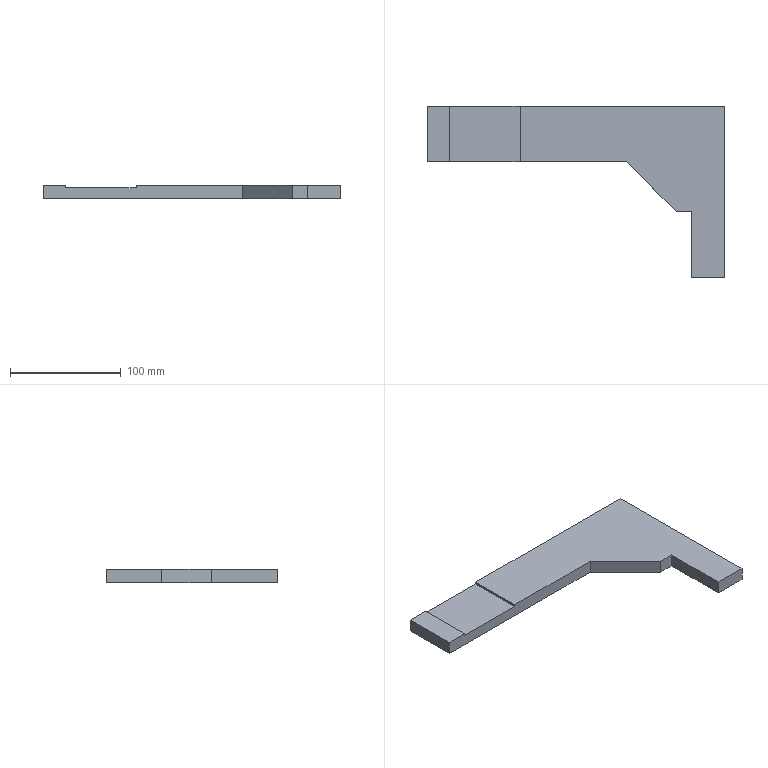Part | SolidWorks | features Cut 1, Extrusion 1 | 1 solid | 14 faces | box 269 x 155 x 12 mm | volume 212510 mm3 | plane 14
STEP:
#1=CARTESIAN_POINT('',(-219.,155.,4.));
#2=VERTEX_POINT('',#1);
#3=CARTESIAN_POINT('',(-219.,155.,6.));
#4=VERTEX_POINT('',#3);
#5=CARTESIAN_POINT('',(-219.,155.,4.));
#6=DIRECTION('',(0.,0.,1.));
#7=VECTOR('',#6,1000.);
#8=LINE('',#5,#7);
#9=EDGE_CURVE('',#2,#4,#8,.T.);
#10=ORIENTED_EDGE('',*,*,#9,.F.);
#11=CARTESIAN_POINT('',(-155.,155.,4.));
#12=VERTEX_POINT('',#11);
#13=CARTESIAN_POINT('',(-219.,155.,4.));
#14=DIRECTION('',(1.,0.,0.));
#15=VECTOR('',#14,1000.);
#16=LINE('',#13,#15);
#17=EDGE_CURVE('',#2,#12,#16,.T.);
#18=ORIENTED_EDGE('',*,*,#17,.T.);
#19=CARTESIAN_POINT('',(-155.,155.,6.));
#20=VERTEX_POINT('',#19);
#21=CARTESIAN_POINT('',(-155.,155.,4.));
#22=DIRECTION('',(0.,0.,1.));
#23=VECTOR('',#22,1000.);
#24=LINE('',#21,#23);
#25=EDGE_CURVE('',#12,#20,#24,.T.);
#26=ORIENTED_EDGE('',*,*,#25,.T.);
#27=CARTESIAN_POINT('',(30.,155.,6.));
#28=VERTEX_POINT('',#27);
#29=CARTESIAN_POINT('',(-239.,155.,6.));
#30=DIRECTION('',(-1.,0.,0.));
#31=VECTOR('',#30,1000.);
#32=LINE('',#29,#31);
#33=EDGE_CURVE('',#28,#20,#32,.T.);
#34=ORIENTED_EDGE('',*,*,#33,.F.);
#35=CARTESIAN_POINT('',(30.,155.,-6.));
#36=VERTEX_POINT('',#35);
#37=CARTESIAN_POINT('',(30.,155.,6.));
#38=DIRECTION('',(0.,0.,-1.));
#39=VECTOR('',#38,1000.);
#40=LINE('',#37,#39);
#41=EDGE_CURVE('',#28,#36,#40,.T.);
#42=ORIENTED_EDGE('',*,*,#41,.T.);
#43=CARTESIAN_POINT('',(-239.,155.,-6.));
#44=VERTEX_POINT('',#43);
#45=CARTESIAN_POINT('',(-239.,155.,-6.));
#46=DIRECTION('',(-1.,0.,0.));
#47=VECTOR('',#46,1000.);
#48=LINE('',#45,#47);
#49=EDGE_CURVE('',#36,#44,#48,.T.);
#50=ORIENTED_EDGE('',*,*,#49,.T.);
#51=CARTESIAN_POINT('',(-239.,155.,6.));
#52=VERTEX_POINT('',#51);
#53=CARTESIAN_POINT('',(-239.,155.,6.));
#54=DIRECTION('',(0.,0.,-1.));
#55=VECTOR('',#54,1000.);
#56=LINE('',#53,#55);
#57=EDGE_CURVE('',#52,#44,#56,.T.);
#58=ORIENTED_EDGE('',*,*,#57,.F.);
#59=CARTESIAN_POINT('',(-239.,155.,6.));
#60=DIRECTION('',(-1.,0.,0.));
#61=VECTOR('',#60,1000.);
#62=LINE('',#59,#61);
#63=EDGE_CURVE('',#4,#52,#62,.T.);
#64=ORIENTED_EDGE('',*,*,#63,.F.);
#65=EDGE_LOOP('',(#10,#18,#26,#34,#42,#50,#58,#64));
#66=FACE_OUTER_BOUND('',#65,.T.);
#67=CARTESIAN_POINT('',(-239.,155.,6.));
#68=DIRECTION('',(0.,-1.,0.));
#69=DIRECTION('',(0.,0.,-1.));
#70=AXIS2_PLACEMENT_3D('',#67,#68,#69);
#71=PLANE('',#70);
#72=ADVANCED_FACE('',(#66),#71,.F.);
#73=CARTESIAN_POINT('',(-219.,105.,4.));
#74=VERTEX_POINT('',#73);
#75=CARTESIAN_POINT('',(-219.,105.,6.));
#76=VERTEX_POINT('',#75);
#77=CARTESIAN_POINT('',(-219.,105.,4.));
#78=DIRECTION('',(0.,0.,1.));
#79=VECTOR('',#78,1000.);
#80=LINE('',#77,#79);
#81=EDGE_CURVE('',#74,#76,#80,.T.);
#82=ORIENTED_EDGE('',*,*,#81,.T.);
#83=CARTESIAN_POINT('',(-239.,105.,6.));
#84=VERTEX_POINT('',#83);
#85=CARTESIAN_POINT('',(-59.,105.,6.));
#86=DIRECTION('',(1.,0.,0.));
#87=VECTOR('',#86,1000.);
#88=LINE('',#85,#87);
#89=EDGE_CURVE('',#84,#76,#88,.T.);
#90=ORIENTED_EDGE('',*,*,#89,.F.);
#91=CARTESIAN_POINT('',(-239.,105.,-6.));
#92=VERTEX_POINT('',#91);
#93=CARTESIAN_POINT('',(-239.,105.,6.));
#94=DIRECTION('',(0.,0.,-1.));
#95=VECTOR('',#94,1000.);
#96=LINE('',#93,#95);
#97=EDGE_CURVE('',#84,#92,#96,.T.);
#98=ORIENTED_EDGE('',*,*,#97,.T.);
#99=CARTESIAN_POINT('',(-59.,105.,-6.));
#100=VERTEX_POINT('',#99);
#101=CARTESIAN_POINT('',(-59.,105.,-6.));
#102=DIRECTION('',(1.,0.,0.));
#103=VECTOR('',#102,1000.);
#104=LINE('',#101,#103);
#105=EDGE_CURVE('',#92,#100,#104,.T.);
#106=ORIENTED_EDGE('',*,*,#105,.T.);
#107=CARTESIAN_POINT('',(-59.,105.,6.));
#108=VERTEX_POINT('',#107);
#109=CARTESIAN_POINT('',(-59.,105.,6.));
#110=DIRECTION('',(0.,0.,-1.));
#111=VECTOR('',#110,1000.);
#112=LINE('',#109,#111);
#113=EDGE_CURVE('',#108,#100,#112,.T.);
#114=ORIENTED_EDGE('',*,*,#113,.F.);
#115=CARTESIAN_POINT('',(-155.,105.,6.));
#116=VERTEX_POINT('',#115);
#117=CARTESIAN_POINT('',(-59.,105.,6.));
#118=DIRECTION('',(1.,0.,0.));
#119=VECTOR('',#118,1000.);
#120=LINE('',#117,#119);
#121=EDGE_CURVE('',#116,#108,#120,.T.);
#122=ORIENTED_EDGE('',*,*,#121,.F.);
#123=CARTESIAN_POINT('',(-155.,105.,4.));
#124=VERTEX_POINT('',#123);
#125=CARTESIAN_POINT('',(-155.,105.,4.));
#126=DIRECTION('',(0.,0.,1.));
#127=VECTOR('',#126,1000.);
#128=LINE('',#125,#127);
#129=EDGE_CURVE('',#124,#116,#128,.T.);
#130=ORIENTED_EDGE('',*,*,#129,.F.);
#131=CARTESIAN_POINT('',(-219.,105.,4.));
#132=DIRECTION('',(-1.,0.,0.));
#133=VECTOR('',#132,1000.);
#134=LINE('',#131,#133);
#135=EDGE_CURVE('',#124,#74,#134,.T.);
#136=ORIENTED_EDGE('',*,*,#135,.T.);
#137=EDGE_LOOP('',(#82,#90,#98,#106,#114,#122,#130,#136));
#138=FACE_OUTER_BOUND('',#137,.T.);
#139=CARTESIAN_POINT('',(-59.,105.,6.));
#140=DIRECTION('',(0.,1.,0.));
#141=DIRECTION('',(-1.,0.,0.));
#142=AXIS2_PLACEMENT_3D('',#139,#140,#141);
#143=PLANE('',#142);
#144=ADVANCED_FACE('',(#138),#143,.F.);
#145=CARTESIAN_POINT('',(-219.,155.,6.));
#146=DIRECTION('',(0.,1.,0.));
#147=VECTOR('',#146,1000.);
#148=LINE('',#145,#147);
#149=EDGE_CURVE('',#76,#4,#148,.T.);
#150=ORIENTED_EDGE('',*,*,#149,.T.);
#151=ORIENTED_EDGE('',*,*,#63,.T.);
#152=CARTESIAN_POINT('',(-239.,105.,6.));
#153=DIRECTION('',(0.,-1.,0.));
#154=VECTOR('',#153,1000.);
#155=LINE('',#152,#154);
#156=EDGE_CURVE('',#52,#84,#155,.T.);
#157=ORIENTED_EDGE('',*,*,#156,.T.);
#158=ORIENTED_EDGE('',*,*,#89,.T.);
#159=EDGE_LOOP('',(#150,#151,#157,#158));
#160=FACE_OUTER_BOUND('',#159,.T.);
#161=CARTESIAN_POINT('',(0.,0.,6.));
#162=DIRECTION('',(0.,0.,-1.));
#163=DIRECTION('',(-1.,0.,0.));
#164=AXIS2_PLACEMENT_3D('',#161,#162,#163);
#165=PLANE('',#164);
#166=ADVANCED_FACE('',(#160),#165,.F.);
#167=CARTESIAN_POINT('',(-155.,155.,6.));
#168=DIRECTION('',(0.,-1.,0.));
#169=VECTOR('',#168,1000.);
#170=LINE('',#167,#169);
#171=EDGE_CURVE('',#20,#116,#170,.T.);
#172=ORIENTED_EDGE('',*,*,#171,.T.);
#173=ORIENTED_EDGE('',*,*,#121,.T.);
#174=CARTESIAN_POINT('',(-14.,60.,6.));
#175=VERTEX_POINT('',#174);
#176=CARTESIAN_POINT('',(-14.,60.,6.));
#177=DIRECTION('',(0.7071,-0.7071,0.));
#178=VECTOR('',#177,1000.);
#179=LINE('',#176,#178);
#180=EDGE_CURVE('',#108,#175,#179,.T.);
#181=ORIENTED_EDGE('',*,*,#180,.T.);
#182=CARTESIAN_POINT('',(0.,60.,6.));
#183=VERTEX_POINT('',#182);
#184=CARTESIAN_POINT('',(0.,60.,6.));
#185=DIRECTION('',(1.,0.,0.));
#186=VECTOR('',#185,1000.);
#187=LINE('',#184,#186);
#188=EDGE_CURVE('',#175,#183,#187,.T.);
#189=ORIENTED_EDGE('',*,*,#188,.T.);
#190=CARTESIAN_POINT('',(0.,0.,6.));
#191=VERTEX_POINT('',#190);
#192=CARTESIAN_POINT('',(0.,0.,6.));
#193=DIRECTION('',(0.,-1.,0.));
#194=VECTOR('',#193,1000.);
#195=LINE('',#192,#194);
#196=EDGE_CURVE('',#183,#191,#195,.T.);
#197=ORIENTED_EDGE('',*,*,#196,.T.);
#198=CARTESIAN_POINT('',(30.,0.,6.));
#199=VERTEX_POINT('',#198);
#200=CARTESIAN_POINT('',(0.,0.,6.));
#201=DIRECTION('',(1.,0.,0.));
#202=VECTOR('',#201,1000.);
#203=LINE('',#200,#202);
#204=EDGE_CURVE('',#191,#199,#203,.T.);
#205=ORIENTED_EDGE('',*,*,#204,.T.);
#206=CARTESIAN_POINT('',(30.,155.,6.));
#207=DIRECTION('',(0.,1.,0.));
#208=VECTOR('',#207,1000.);
#209=LINE('',#206,#208);
#210=EDGE_CURVE('',#199,#28,#209,.T.);
#211=ORIENTED_EDGE('',*,*,#210,.T.);
#212=ORIENTED_EDGE('',*,*,#33,.T.);
#213=EDGE_LOOP('',(#172,#173,#181,#189,#197,#205,#211,#212));
#214=FACE_OUTER_BOUND('',#213,.T.);
#215=CARTESIAN_POINT('',(0.,0.,6.));
#216=DIRECTION('',(0.,0.,-1.));
#217=DIRECTION('',(-1.,0.,0.));
#218=AXIS2_PLACEMENT_3D('',#215,#216,#217);
#219=PLANE('',#218);
#220=ADVANCED_FACE('',(#214),#219,.F.);
#221=CARTESIAN_POINT('',(0.,0.,-6.));
#222=VERTEX_POINT('',#221);
#223=CARTESIAN_POINT('',(30.,0.,-6.));
#224=VERTEX_POINT('',#223);
#225=CARTESIAN_POINT('',(0.,0.,-6.));
#226=DIRECTION('',(1.,0.,0.));
#227=VECTOR('',#226,1000.);
#228=LINE('',#225,#227);
#229=EDGE_CURVE('',#222,#224,#228,.T.);
#230=ORIENTED_EDGE('',*,*,#229,.T.);
#231=CARTESIAN_POINT('',(30.,0.,6.));
#232=DIRECTION('',(0.,0.,-1.));
#233=VECTOR('',#232,1000.);
#234=LINE('',#231,#233);
#235=EDGE_CURVE('',#199,#224,#234,.T.);
#236=ORIENTED_EDGE('',*,*,#235,.F.);
#237=ORIENTED_EDGE('',*,*,#204,.F.);
#238=CARTESIAN_POINT('',(0.,0.,6.));
#239=DIRECTION('',(0.,0.,-1.));
#240=VECTOR('',#239,1000.);
#241=LINE('',#238,#240);
#242=EDGE_CURVE('',#191,#222,#241,.T.);
#243=ORIENTED_EDGE('',*,*,#242,.T.);
#244=EDGE_LOOP('',(#230,#236,#237,#243));
#245=FACE_OUTER_BOUND('',#244,.T.);
#246=CARTESIAN_POINT('',(0.,0.,6.));
#247=DIRECTION('',(0.,1.,0.));
#248=DIRECTION('',(0.,0.,1.));
#249=AXIS2_PLACEMENT_3D('',#246,#247,#248);
#250=PLANE('',#249);
#251=ADVANCED_FACE('',(#245),#250,.F.);
#252=CARTESIAN_POINT('',(30.,155.,-6.));
#253=DIRECTION('',(0.,1.,0.));
#254=VECTOR('',#253,1000.);
#255=LINE('',#252,#254);
#256=EDGE_CURVE('',#224,#36,#255,.T.);
#257=ORIENTED_EDGE('',*,*,#256,.T.);
#258=ORIENTED_EDGE('',*,*,#41,.F.);
#259=ORIENTED_EDGE('',*,*,#210,.F.);
#260=ORIENTED_EDGE('',*,*,#235,.T.);
#261=EDGE_LOOP('',(#257,#258,#259,#260));
#262=FACE_OUTER_BOUND('',#261,.T.);
#263=CARTESIAN_POINT('',(30.,155.,6.));
#264=DIRECTION('',(-1.,0.,0.));
#265=DIRECTION('',(0.,0.,1.));
#266=AXIS2_PLACEMENT_3D('',#263,#264,#265);
#267=PLANE('',#266);
#268=ADVANCED_FACE('',(#262),#267,.F.);
#269=CARTESIAN_POINT('',(-239.,105.,-6.));
#270=DIRECTION('',(0.,-1.,0.));
#271=VECTOR('',#270,1000.);
#272=LINE('',#269,#271);
#273=EDGE_CURVE('',#44,#92,#272,.T.);
#274=ORIENTED_EDGE('',*,*,#273,.T.);
#275=ORIENTED_EDGE('',*,*,#97,.F.);
#276=ORIENTED_EDGE('',*,*,#156,.F.);
#277=ORIENTED_EDGE('',*,*,#57,.T.);
#278=EDGE_LOOP('',(#274,#275,#276,#277));
#279=FACE_OUTER_BOUND('',#278,.T.);
#280=CARTESIAN_POINT('',(-239.,105.,6.));
#281=DIRECTION('',(1.,0.,0.));
#282=DIRECTION('',(0.,1.,0.));
#283=AXIS2_PLACEMENT_3D('',#280,#281,#282);
#284=PLANE('',#283);
#285=ADVANCED_FACE('',(#279),#284,.F.);
#286=CARTESIAN_POINT('',(-14.,60.,-6.));
#287=VERTEX_POINT('',#286);
#288=CARTESIAN_POINT('',(-14.,60.,-6.));
#289=DIRECTION('',(0.7071,-0.7071,0.));
#290=VECTOR('',#289,1000.);
#291=LINE('',#288,#290);
#292=EDGE_CURVE('',#100,#287,#291,.T.);
#293=ORIENTED_EDGE('',*,*,#292,.T.);
#294=CARTESIAN_POINT('',(-14.,60.,6.));
#295=DIRECTION('',(0.,0.,-1.));
#296=VECTOR('',#295,1000.);
#297=LINE('',#294,#296);
#298=EDGE_CURVE('',#175,#287,#297,.T.);
#299=ORIENTED_EDGE('',*,*,#298,.F.);
#300=ORIENTED_EDGE('',*,*,#180,.F.);
#301=ORIENTED_EDGE('',*,*,#113,.T.);
#302=EDGE_LOOP('',(#293,#299,#300,#301));
#303=FACE_OUTER_BOUND('',#302,.T.);
#304=CARTESIAN_POINT('',(-14.,60.,6.));
#305=DIRECTION('',(0.7071,0.7071,0.));
#306=DIRECTION('',(-0.7071,0.7071,0.));
#307=AXIS2_PLACEMENT_3D('',#304,#305,#306);
#308=PLANE('',#307);
#309=ADVANCED_FACE('',(#303),#308,.F.);
#310=CARTESIAN_POINT('',(0.,60.,-6.));
#311=VERTEX_POINT('',#310);
#312=CARTESIAN_POINT('',(0.,60.,-6.));
#313=DIRECTION('',(1.,0.,0.));
#314=VECTOR('',#313,1000.);
#315=LINE('',#312,#314);
#316=EDGE_CURVE('',#287,#311,#315,.T.);
#317=ORIENTED_EDGE('',*,*,#316,.T.);
#318=CARTESIAN_POINT('',(0.,60.,6.));
#319=DIRECTION('',(0.,0.,-1.));
#320=VECTOR('',#319,1000.);
#321=LINE('',#318,#320);
#322=EDGE_CURVE('',#183,#311,#321,.T.);
#323=ORIENTED_EDGE('',*,*,#322,.F.);
#324=ORIENTED_EDGE('',*,*,#188,.F.);
#325=ORIENTED_EDGE('',*,*,#298,.T.);
#326=EDGE_LOOP('',(#317,#323,#324,#325));
#327=FACE_OUTER_BOUND('',#326,.T.);
#328=CARTESIAN_POINT('',(0.,60.,6.));
#329=DIRECTION('',(0.,1.,0.));
#330=DIRECTION('',(0.,0.,1.));
#331=AXIS2_PLACEMENT_3D('',#328,#329,#330);
#332=PLANE('',#331);
#333=ADVANCED_FACE('',(#327),#332,.F.);
#334=CARTESIAN_POINT('',(0.,0.,-6.));
#335=DIRECTION('',(0.,-1.,0.));
#336=VECTOR('',#335,1000.);
#337=LINE('',#334,#336);
#338=EDGE_CURVE('',#311,#222,#337,.T.);
#339=ORIENTED_EDGE('',*,*,#338,.T.);
#340=ORIENTED_EDGE('',*,*,#242,.F.);
#341=ORIENTED_EDGE('',*,*,#196,.F.);
#342=ORIENTED_EDGE('',*,*,#322,.T.);
#343=EDGE_LOOP('',(#339,#340,#341,#342));
#344=FACE_OUTER_BOUND('',#343,.T.);
#345=CARTESIAN_POINT('',(0.,0.,6.));
#346=DIRECTION('',(1.,0.,0.));
#347=DIRECTION('',(0.,0.,-1.));
#348=AXIS2_PLACEMENT_3D('',#345,#346,#347);
#349=PLANE('',#348);
#350=ADVANCED_FACE('',(#344),#349,.F.);
#351=ORIENTED_EDGE('',*,*,#229,.F.);
#352=ORIENTED_EDGE('',*,*,#338,.F.);
#353=ORIENTED_EDGE('',*,*,#316,.F.);
#354=ORIENTED_EDGE('',*,*,#292,.F.);
#355=ORIENTED_EDGE('',*,*,#105,.F.);
#356=ORIENTED_EDGE('',*,*,#273,.F.);
#357=ORIENTED_EDGE('',*,*,#49,.F.);
#358=ORIENTED_EDGE('',*,*,#256,.F.);
#359=EDGE_LOOP('',(#351,#352,#353,#354,#355,#356,#357,#358));
#360=FACE_OUTER_BOUND('',#359,.T.);
#361=CARTESIAN_POINT('',(0.,0.,-6.));
#362=DIRECTION('',(0.,0.,-1.));
#363=DIRECTION('',(-1.,0.,0.));
#364=AXIS2_PLACEMENT_3D('',#361,#362,#363);
#365=PLANE('',#364);
#366=ADVANCED_FACE('',(#360),#365,.T.);
#367=ORIENTED_EDGE('',*,*,#149,.F.);
#368=ORIENTED_EDGE('',*,*,#81,.F.);
#369=CARTESIAN_POINT('',(-219.,155.,4.));
#370=DIRECTION('',(0.,1.,0.));
#371=VECTOR('',#370,1000.);
#372=LINE('',#369,#371);
#373=EDGE_CURVE('',#74,#2,#372,.T.);
#374=ORIENTED_EDGE('',*,*,#373,.T.);
#375=ORIENTED_EDGE('',*,*,#9,.T.);
#376=EDGE_LOOP('',(#367,#368,#374,#375));
#377=FACE_OUTER_BOUND('',#376,.T.);
#378=CARTESIAN_POINT('',(-219.,155.,4.));
#379=DIRECTION('',(1.,0.,0.));
#380=DIRECTION('',(0.,0.,-1.));
#381=AXIS2_PLACEMENT_3D('',#378,#379,#380);
#382=PLANE('',#381);
#383=ADVANCED_FACE('',(#377),#382,.T.);
#384=ORIENTED_EDGE('',*,*,#171,.F.);
#385=ORIENTED_EDGE('',*,*,#25,.F.);
#386=CARTESIAN_POINT('',(-155.,155.,4.));
#387=DIRECTION('',(0.,-1.,0.));
#388=VECTOR('',#387,1000.);
#389=LINE('',#386,#388);
#390=EDGE_CURVE('',#12,#124,#389,.T.);
#391=ORIENTED_EDGE('',*,*,#390,.T.);
#392=ORIENTED_EDGE('',*,*,#129,.T.);
#393=EDGE_LOOP('',(#384,#385,#391,#392));
#394=FACE_OUTER_BOUND('',#393,.T.);
#395=CARTESIAN_POINT('',(-155.,155.,4.));
#396=DIRECTION('',(-1.,0.,0.));
#397=DIRECTION('',(0.,-1.,0.));
#398=AXIS2_PLACEMENT_3D('',#395,#396,#397);
#399=PLANE('',#398);
#400=ADVANCED_FACE('',(#394),#399,.T.);
#401=ORIENTED_EDGE('',*,*,#373,.F.);
#402=ORIENTED_EDGE('',*,*,#135,.F.);
#403=ORIENTED_EDGE('',*,*,#390,.F.);
#404=ORIENTED_EDGE('',*,*,#17,.F.);
#405=EDGE_LOOP('',(#401,#402,#403,#404));
#406=FACE_OUTER_BOUND('',#405,.T.);
#407=CARTESIAN_POINT('',(0.,0.,4.));
#408=DIRECTION('',(0.,0.,1.));
#409=DIRECTION('',(1.,0.,0.));
#410=AXIS2_PLACEMENT_3D('',#407,#408,#409);
#411=PLANE('',#410);
#412=ADVANCED_FACE('',(#406),#411,.T.);
#413=CLOSED_SHELL('',(#72,#144,#166,#220,#251,#268,#285,#309,#333,#350,#366,#383,#400,#412));
#414=MANIFOLD_SOLID_BREP('',#413);
#415=CARTESIAN_POINT('',(0.,0.,0.));
#416=DIRECTION('',(0.,0.,1.));
#417=DIRECTION('',(1.,0.,0.));
#418=AXIS2_PLACEMENT_3D('',#415,#416,#417);
#419=(LENGTH_UNIT()NAMED_UNIT(*)SI_UNIT(.MILLI.,.METRE.));
#420=UNCERTAINTY_MEASURE_WITH_UNIT(LENGTH_MEASURE(0.00001),#419,'','');
#421=(NAMED_UNIT(*)PLANE_ANGLE_UNIT()SI_UNIT($,.RADIAN.));
#422=(NAMED_UNIT(*)SI_UNIT($,.STERADIAN.)SOLID_ANGLE_UNIT());
#423=(GEOMETRIC_REPRESENTATION_CONTEXT(3)GLOBAL_UNCERTAINTY_ASSIGNED_CONTEXT((#420))GLOBAL_UNIT_ASSIGNED_CONTEXT((#419,#421,#422))REPRESENTATION_CONTEXT('',''));
#424=ADVANCED_BREP_SHAPE_REPRESENTATION('',(#414,#418),#423);